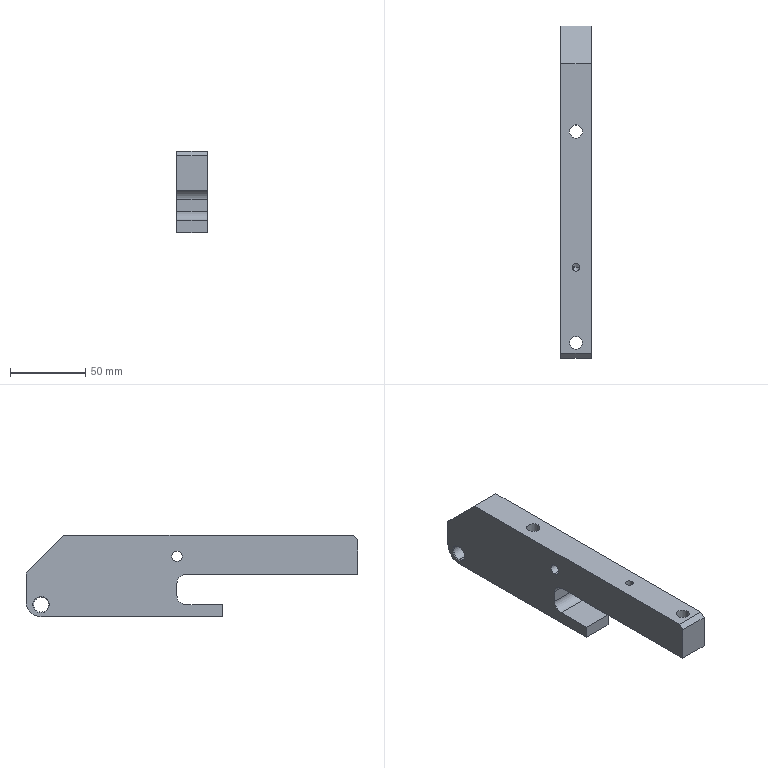Part | STEP file | 0217_202_Arm | 1 solid | 31 faces | box 20 x 220 x 54 mm | volume 161429 mm3 | cylinder 13 | plane 12 | cone 6 | commonest cylinder face diameters 5 x2 6.8 x2 8.5 x2 8.8 x2 10 x2 12 x2